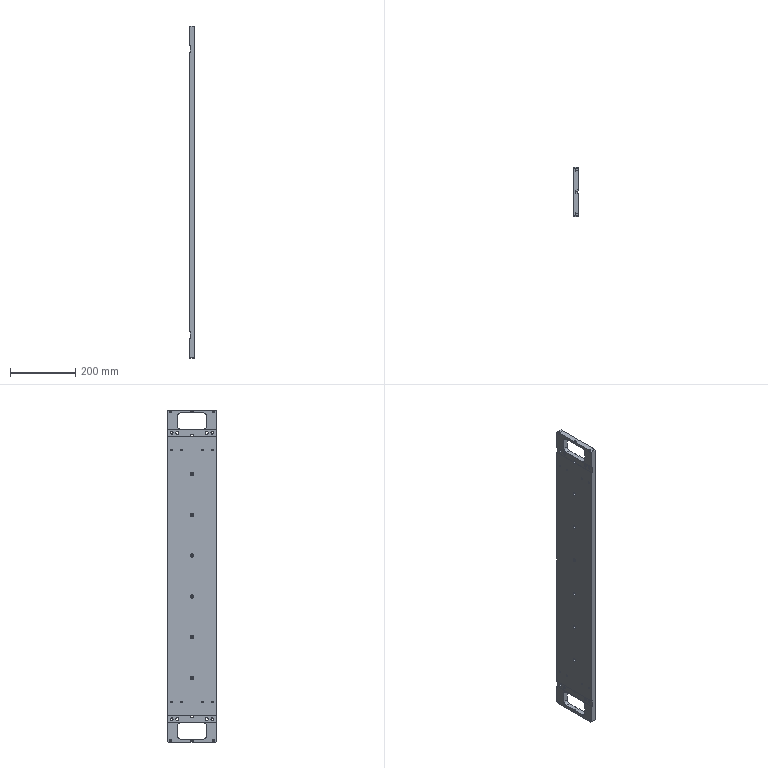Part | SolidWorks | features HoleWzd 6, ICE 3, MirrorPattern 2, Chamfer 1, Extrusion 1, Fillet 1 | 1 solid | 154 faces | box 15 x 150 x 1018 mm | volume 2102309 mm3 | cylinder 100 | plane 54 | commonest cylinder face diameters 8 x24 5 x16 4.3 x12 6.6 x12 11 x12 9 x8